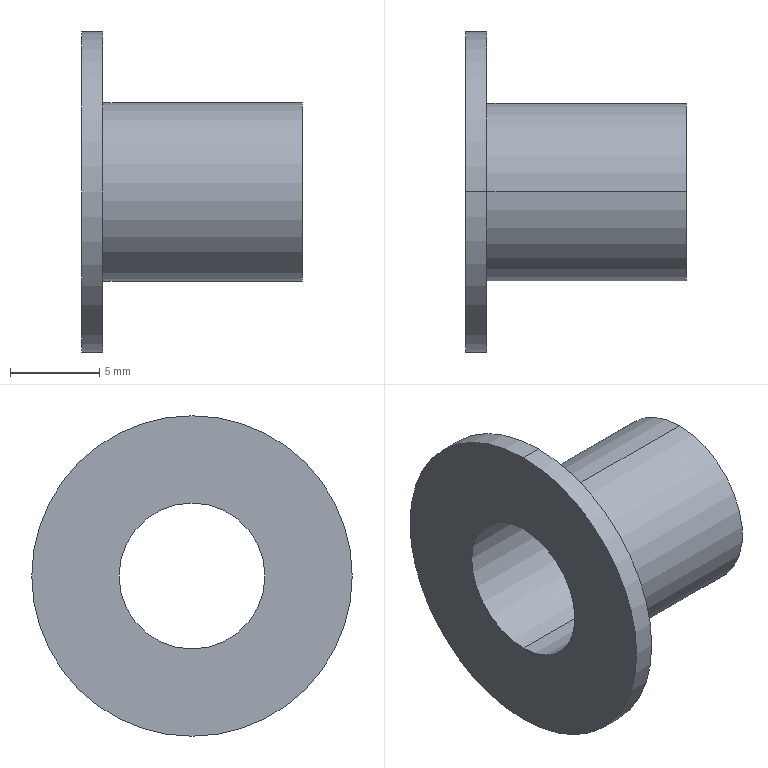Part | SolidWorks | features Revolution 1 | 1 solid | 9 faces | box 12.4 x 18 x 18 mm | volume 530.163 mm3 | cylinder 6 | plane 3 | commonest cylinder face diameters 8.2 x2 10 x2 18 x2
STEP:
#1=CARTESIAN_POINT('',(12.4,0.,5.));
#2=VERTEX_POINT('',#1);
#3=CARTESIAN_POINT('',(12.4,0.,-5.));
#4=VERTEX_POINT('',#3);
#5=CARTESIAN_POINT('',(12.4,0.,0.));
#6=DIRECTION('',(-1.,0.,0.));
#7=DIRECTION('',(0.,0.,1.));
#8=AXIS2_PLACEMENT_3D('',#5,#6,#7);
#9=CIRCLE('',#8,5.);
#10=EDGE_CURVE('',#2,#4,#9,.T.);
#11=ORIENTED_EDGE('',*,*,#10,.T.);
#12=CARTESIAN_POINT('',(1.2,0.,-5.));
#13=VERTEX_POINT('',#12);
#14=CARTESIAN_POINT('',(0.,0.,-5.));
#15=DIRECTION('',(-1.,0.,0.));
#16=VECTOR('',#15,1000.);
#17=LINE('',#14,#16);
#18=EDGE_CURVE('',#4,#13,#17,.T.);
#19=ORIENTED_EDGE('',*,*,#18,.T.);
#20=CARTESIAN_POINT('',(1.2,0.,5.));
#21=VERTEX_POINT('',#20);
#22=CARTESIAN_POINT('',(1.2,0.,0.));
#23=DIRECTION('',(-1.,0.,0.));
#24=DIRECTION('',(0.,0.,1.));
#25=AXIS2_PLACEMENT_3D('',#22,#23,#24);
#26=CIRCLE('',#25,5.);
#27=EDGE_CURVE('',#21,#13,#26,.T.);
#28=ORIENTED_EDGE('',*,*,#27,.F.);
#29=CARTESIAN_POINT('',(0.,0.,5.));
#30=DIRECTION('',(-1.,0.,0.));
#31=VECTOR('',#30,1000.);
#32=LINE('',#29,#31);
#33=EDGE_CURVE('',#2,#21,#32,.T.);
#34=ORIENTED_EDGE('',*,*,#33,.F.);
#35=EDGE_LOOP('',(#11,#19,#28,#34));
#36=FACE_OUTER_BOUND('',#35,.T.);
#37=CARTESIAN_POINT('',(0.,0.,0.));
#38=DIRECTION('',(-1.,0.,0.));
#39=DIRECTION('',(0.,0.,1.));
#40=AXIS2_PLACEMENT_3D('',#37,#38,#39);
#41=CYLINDRICAL_SURFACE('',#40,5.);
#42=ADVANCED_FACE('',(#36),#41,.T.);
#43=CARTESIAN_POINT('',(12.4,0.,-4.1));
#44=VERTEX_POINT('',#43);
#45=CARTESIAN_POINT('',(12.4,0.,4.1));
#46=VERTEX_POINT('',#45);
#47=CARTESIAN_POINT('',(12.4,0.,0.));
#48=DIRECTION('',(-1.,0.,0.));
#49=DIRECTION('',(0.,0.,1.));
#50=AXIS2_PLACEMENT_3D('',#47,#48,#49);
#51=CIRCLE('',#50,4.1);
#52=EDGE_CURVE('',#44,#46,#51,.T.);
#53=ORIENTED_EDGE('',*,*,#52,.F.);
#54=CARTESIAN_POINT('',(0.,0.,-4.1));
#55=VERTEX_POINT('',#54);
#56=CARTESIAN_POINT('',(0.,0.,-4.1));
#57=DIRECTION('',(-1.,0.,0.));
#58=VECTOR('',#57,1000.);
#59=LINE('',#56,#58);
#60=EDGE_CURVE('',#44,#55,#59,.T.);
#61=ORIENTED_EDGE('',*,*,#60,.T.);
#62=CARTESIAN_POINT('',(0.,0.,4.1));
#63=VERTEX_POINT('',#62);
#64=CARTESIAN_POINT('',(0.,0.,0.));
#65=DIRECTION('',(-1.,0.,0.));
#66=DIRECTION('',(0.,0.,1.));
#67=AXIS2_PLACEMENT_3D('',#64,#65,#66);
#68=CIRCLE('',#67,4.1);
#69=EDGE_CURVE('',#55,#63,#68,.T.);
#70=ORIENTED_EDGE('',*,*,#69,.T.);
#71=CARTESIAN_POINT('',(0.,0.,4.1));
#72=DIRECTION('',(-1.,0.,0.));
#73=VECTOR('',#72,1000.);
#74=LINE('',#71,#73);
#75=EDGE_CURVE('',#46,#63,#74,.T.);
#76=ORIENTED_EDGE('',*,*,#75,.F.);
#77=EDGE_LOOP('',(#53,#61,#70,#76));
#78=FACE_OUTER_BOUND('',#77,.T.);
#79=CARTESIAN_POINT('',(0.,0.,0.));
#80=DIRECTION('',(-1.,0.,0.));
#81=DIRECTION('',(0.,0.,1.));
#82=AXIS2_PLACEMENT_3D('',#79,#80,#81);
#83=CYLINDRICAL_SURFACE('',#82,4.1);
#84=ADVANCED_FACE('',(#78),#83,.F.);
#85=CARTESIAN_POINT('',(1.2,0.,9.));
#86=VERTEX_POINT('',#85);
#87=CARTESIAN_POINT('',(1.2,0.,-9.));
#88=VERTEX_POINT('',#87);
#89=CARTESIAN_POINT('',(1.2,0.,0.));
#90=DIRECTION('',(-1.,0.,0.));
#91=DIRECTION('',(0.,0.,1.));
#92=AXIS2_PLACEMENT_3D('',#89,#90,#91);
#93=CIRCLE('',#92,9.);
#94=EDGE_CURVE('',#86,#88,#93,.T.);
#95=ORIENTED_EDGE('',*,*,#94,.T.);
#96=CARTESIAN_POINT('',(0.,0.,-9.));
#97=VERTEX_POINT('',#96);
#98=CARTESIAN_POINT('',(0.,0.,-9.));
#99=DIRECTION('',(-1.,0.,0.));
#100=VECTOR('',#99,1000.);
#101=LINE('',#98,#100);
#102=EDGE_CURVE('',#88,#97,#101,.T.);
#103=ORIENTED_EDGE('',*,*,#102,.T.);
#104=CARTESIAN_POINT('',(0.,0.,9.));
#105=VERTEX_POINT('',#104);
#106=CARTESIAN_POINT('',(0.,0.,0.));
#107=DIRECTION('',(-1.,0.,0.));
#108=DIRECTION('',(0.,0.,1.));
#109=AXIS2_PLACEMENT_3D('',#106,#107,#108);
#110=CIRCLE('',#109,9.);
#111=EDGE_CURVE('',#105,#97,#110,.T.);
#112=ORIENTED_EDGE('',*,*,#111,.F.);
#113=CARTESIAN_POINT('',(0.,0.,9.));
#114=DIRECTION('',(-1.,0.,0.));
#115=VECTOR('',#114,1000.);
#116=LINE('',#113,#115);
#117=EDGE_CURVE('',#86,#105,#116,.T.);
#118=ORIENTED_EDGE('',*,*,#117,.F.);
#119=EDGE_LOOP('',(#95,#103,#112,#118));
#120=FACE_OUTER_BOUND('',#119,.T.);
#121=CARTESIAN_POINT('',(0.,0.,0.));
#122=DIRECTION('',(-1.,0.,0.));
#123=DIRECTION('',(0.,0.,1.));
#124=AXIS2_PLACEMENT_3D('',#121,#122,#123);
#125=CYLINDRICAL_SURFACE('',#124,9.);
#126=ADVANCED_FACE('',(#120),#125,.T.);
#127=ORIENTED_EDGE('',*,*,#94,.F.);
#128=CARTESIAN_POINT('',(1.2,0.,0.));
#129=DIRECTION('',(-1.,0.,0.));
#130=DIRECTION('',(0.,0.,1.));
#131=AXIS2_PLACEMENT_3D('',#128,#129,#130);
#132=CIRCLE('',#131,9.);
#133=EDGE_CURVE('',#88,#86,#132,.T.);
#134=ORIENTED_EDGE('',*,*,#133,.F.);
#135=EDGE_LOOP('',(#127,#134));
#136=FACE_OUTER_BOUND('',#135,.T.);
#137=ORIENTED_EDGE('',*,*,#27,.T.);
#138=CARTESIAN_POINT('',(1.2,0.,0.));
#139=DIRECTION('',(-1.,0.,0.));
#140=DIRECTION('',(0.,0.,1.));
#141=AXIS2_PLACEMENT_3D('',#138,#139,#140);
#142=CIRCLE('',#141,5.);
#143=EDGE_CURVE('',#13,#21,#142,.T.);
#144=ORIENTED_EDGE('',*,*,#143,.T.);
#145=EDGE_LOOP('',(#137,#144));
#146=FACE_BOUND('',#145,.T.);
#147=CARTESIAN_POINT('',(1.2,9.,0.));
#148=DIRECTION('',(-1.,0.,0.));
#149=DIRECTION('',(0.,0.,1.));
#150=AXIS2_PLACEMENT_3D('',#147,#148,#149);
#151=PLANE('',#150);
#152=ADVANCED_FACE('',(#136,#146),#151,.F.);
#153=ORIENTED_EDGE('',*,*,#102,.F.);
#154=ORIENTED_EDGE('',*,*,#133,.T.);
#155=ORIENTED_EDGE('',*,*,#117,.T.);
#156=CARTESIAN_POINT('',(0.,0.,0.));
#157=DIRECTION('',(-1.,0.,0.));
#158=DIRECTION('',(0.,0.,1.));
#159=AXIS2_PLACEMENT_3D('',#156,#157,#158);
#160=CIRCLE('',#159,9.);
#161=EDGE_CURVE('',#97,#105,#160,.T.);
#162=ORIENTED_EDGE('',*,*,#161,.F.);
#163=EDGE_LOOP('',(#153,#154,#155,#162));
#164=FACE_OUTER_BOUND('',#163,.T.);
#165=CARTESIAN_POINT('',(0.,0.,0.));
#166=DIRECTION('',(-1.,0.,0.));
#167=DIRECTION('',(0.,0.,1.));
#168=AXIS2_PLACEMENT_3D('',#165,#166,#167);
#169=CYLINDRICAL_SURFACE('',#168,9.);
#170=ADVANCED_FACE('',(#164),#169,.T.);
#171=CARTESIAN_POINT('',(0.,0.,0.));
#172=DIRECTION('',(-1.,0.,0.));
#173=DIRECTION('',(0.,0.,1.));
#174=AXIS2_PLACEMENT_3D('',#171,#172,#173);
#175=CIRCLE('',#174,4.1);
#176=EDGE_CURVE('',#63,#55,#175,.T.);
#177=ORIENTED_EDGE('',*,*,#176,.F.);
#178=ORIENTED_EDGE('',*,*,#69,.F.);
#179=EDGE_LOOP('',(#177,#178));
#180=FACE_BOUND('',#179,.T.);
#181=ORIENTED_EDGE('',*,*,#111,.T.);
#182=ORIENTED_EDGE('',*,*,#161,.T.);
#183=EDGE_LOOP('',(#181,#182));
#184=FACE_OUTER_BOUND('',#183,.T.);
#185=CARTESIAN_POINT('',(0.,4.1,0.));
#186=DIRECTION('',(1.,0.,0.));
#187=DIRECTION('',(0.,0.,-1.));
#188=AXIS2_PLACEMENT_3D('',#185,#186,#187);
#189=PLANE('',#188);
#190=ADVANCED_FACE('',(#180,#184),#189,.F.);
#191=ORIENTED_EDGE('',*,*,#60,.F.);
#192=CARTESIAN_POINT('',(12.4,0.,0.));
#193=DIRECTION('',(-1.,0.,0.));
#194=DIRECTION('',(0.,0.,1.));
#195=AXIS2_PLACEMENT_3D('',#192,#193,#194);
#196=CIRCLE('',#195,4.1);
#197=EDGE_CURVE('',#46,#44,#196,.T.);
#198=ORIENTED_EDGE('',*,*,#197,.F.);
#199=ORIENTED_EDGE('',*,*,#75,.T.);
#200=ORIENTED_EDGE('',*,*,#176,.T.);
#201=EDGE_LOOP('',(#191,#198,#199,#200));
#202=FACE_OUTER_BOUND('',#201,.T.);
#203=CARTESIAN_POINT('',(0.,0.,0.));
#204=DIRECTION('',(-1.,0.,0.));
#205=DIRECTION('',(0.,0.,1.));
#206=AXIS2_PLACEMENT_3D('',#203,#204,#205);
#207=CYLINDRICAL_SURFACE('',#206,4.1);
#208=ADVANCED_FACE('',(#202),#207,.F.);
#209=ORIENTED_EDGE('',*,*,#10,.F.);
#210=CARTESIAN_POINT('',(12.4,0.,0.));
#211=DIRECTION('',(-1.,0.,0.));
#212=DIRECTION('',(0.,0.,1.));
#213=AXIS2_PLACEMENT_3D('',#210,#211,#212);
#214=CIRCLE('',#213,5.);
#215=EDGE_CURVE('',#4,#2,#214,.T.);
#216=ORIENTED_EDGE('',*,*,#215,.F.);
#217=EDGE_LOOP('',(#209,#216));
#218=FACE_OUTER_BOUND('',#217,.T.);
#219=ORIENTED_EDGE('',*,*,#197,.T.);
#220=ORIENTED_EDGE('',*,*,#52,.T.);
#221=EDGE_LOOP('',(#219,#220));
#222=FACE_BOUND('',#221,.T.);
#223=CARTESIAN_POINT('',(12.4,5.,0.));
#224=DIRECTION('',(-1.,0.,0.));
#225=DIRECTION('',(0.,0.,1.));
#226=AXIS2_PLACEMENT_3D('',#223,#224,#225);
#227=PLANE('',#226);
#228=ADVANCED_FACE('',(#218,#222),#227,.F.);
#229=ORIENTED_EDGE('',*,*,#18,.F.);
#230=ORIENTED_EDGE('',*,*,#215,.T.);
#231=ORIENTED_EDGE('',*,*,#33,.T.);
#232=ORIENTED_EDGE('',*,*,#143,.F.);
#233=EDGE_LOOP('',(#229,#230,#231,#232));
#234=FACE_OUTER_BOUND('',#233,.T.);
#235=CARTESIAN_POINT('',(0.,0.,0.));
#236=DIRECTION('',(-1.,0.,0.));
#237=DIRECTION('',(0.,0.,1.));
#238=AXIS2_PLACEMENT_3D('',#235,#236,#237);
#239=CYLINDRICAL_SURFACE('',#238,5.);
#240=ADVANCED_FACE('',(#234),#239,.T.);
#241=CLOSED_SHELL('',(#42,#84,#126,#152,#170,#190,#208,#228,#240));
#242=MANIFOLD_SOLID_BREP('',#241);
#243=CARTESIAN_POINT('',(0.,0.,0.));
#244=DIRECTION('',(0.,0.,1.));
#245=DIRECTION('',(1.,0.,0.));
#246=AXIS2_PLACEMENT_3D('',#243,#244,#245);
#247=(LENGTH_UNIT()NAMED_UNIT(*)SI_UNIT(.MILLI.,.METRE.));
#248=UNCERTAINTY_MEASURE_WITH_UNIT(LENGTH_MEASURE(0.00001),#247,'','');
#249=(NAMED_UNIT(*)PLANE_ANGLE_UNIT()SI_UNIT($,.RADIAN.));
#250=(NAMED_UNIT(*)SI_UNIT($,.STERADIAN.)SOLID_ANGLE_UNIT());
#251=(GEOMETRIC_REPRESENTATION_CONTEXT(3)GLOBAL_UNCERTAINTY_ASSIGNED_CONTEXT((#248))GLOBAL_UNIT_ASSIGNED_CONTEXT((#247,#249,#250))REPRESENTATION_CONTEXT('',''));
#252=ADVANCED_BREP_SHAPE_REPRESENTATION('',(#242,#246),#251);